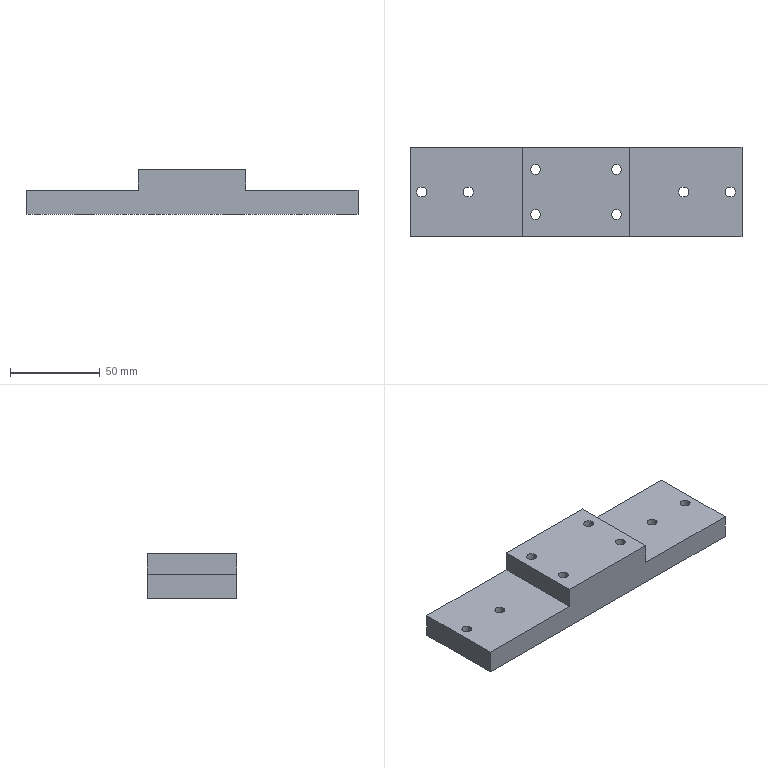Part | SolidWorks | features HoleWzd 2, Extrusion 1, ICE 1 | 1 solid | 50 faces | box 185 x 50 x 25 mm | volume 153218 mm3 | cylinder 32 | plane 18 | commonest cylinder face diameters 5.5 x16 10 x16
STEP:
#1=CARTESIAN_POINT('',(27.5,12.5,5.7));
#2=VERTEX_POINT('',#1);
#3=CARTESIAN_POINT('',(17.5,12.5,5.7));
#4=VERTEX_POINT('',#3);
#5=CARTESIAN_POINT('',(22.5,12.5,5.7));
#6=DIRECTION('',(0.,0.,-1.));
#7=DIRECTION('',(-1.,0.,0.));
#8=AXIS2_PLACEMENT_3D('',#5,#6,#7);
#9=CIRCLE('',#8,5.);
#10=EDGE_CURVE('',#2,#4,#9,.T.);
#11=ORIENTED_EDGE('',*,*,#10,.F.);
#12=CARTESIAN_POINT('',(27.5,12.5,0.));
#13=VERTEX_POINT('',#12);
#14=CARTESIAN_POINT('',(27.5,12.5,0.));
#15=DIRECTION('',(0.,0.,-1.));
#16=VECTOR('',#15,1000.);
#17=LINE('',#14,#16);
#18=EDGE_CURVE('',#2,#13,#17,.T.);
#19=ORIENTED_EDGE('',*,*,#18,.T.);
#20=CARTESIAN_POINT('',(17.5,12.5,0.));
#21=VERTEX_POINT('',#20);
#22=CARTESIAN_POINT('',(22.5,12.5,0.));
#23=DIRECTION('',(0.,0.,-1.));
#24=DIRECTION('',(-1.,0.,0.));
#25=AXIS2_PLACEMENT_3D('',#22,#23,#24);
#26=CIRCLE('',#25,5.);
#27=EDGE_CURVE('',#13,#21,#26,.T.);
#28=ORIENTED_EDGE('',*,*,#27,.T.);
#29=CARTESIAN_POINT('',(17.5,12.5,0.));
#30=DIRECTION('',(0.,0.,-1.));
#31=VECTOR('',#30,1000.);
#32=LINE('',#29,#31);
#33=EDGE_CURVE('',#4,#21,#32,.T.);
#34=ORIENTED_EDGE('',*,*,#33,.F.);
#35=EDGE_LOOP('',(#11,#19,#28,#34));
#36=FACE_OUTER_BOUND('',#35,.T.);
#37=CARTESIAN_POINT('',(22.5,12.5,0.));
#38=DIRECTION('',(0.,0.,-1.));
#39=DIRECTION('',(-1.,0.,0.));
#40=AXIS2_PLACEMENT_3D('',#37,#38,#39);
#41=CYLINDRICAL_SURFACE('',#40,5.);
#42=ADVANCED_FACE('',(#36),#41,.F.);
#43=CARTESIAN_POINT('',(25.25,12.5,25.));
#44=VERTEX_POINT('',#43);
#45=CARTESIAN_POINT('',(19.75,12.5,25.));
#46=VERTEX_POINT('',#45);
#47=CARTESIAN_POINT('',(22.5,12.5,25.));
#48=DIRECTION('',(0.,0.,-1.));
#49=DIRECTION('',(-1.,0.,0.));
#50=AXIS2_PLACEMENT_3D('',#47,#48,#49);
#51=CIRCLE('',#50,2.75);
#52=EDGE_CURVE('',#44,#46,#51,.T.);
#53=ORIENTED_EDGE('',*,*,#52,.F.);
#54=CARTESIAN_POINT('',(25.25,12.5,5.7));
#55=VERTEX_POINT('',#54);
#56=CARTESIAN_POINT('',(25.25,12.5,0.));
#57=DIRECTION('',(0.,0.,-1.));
#58=VECTOR('',#57,1000.);
#59=LINE('',#56,#58);
#60=EDGE_CURVE('',#44,#55,#59,.T.);
#61=ORIENTED_EDGE('',*,*,#60,.T.);
#62=CARTESIAN_POINT('',(19.75,12.5,5.7));
#63=VERTEX_POINT('',#62);
#64=CARTESIAN_POINT('',(22.5,12.5,5.7));
#65=DIRECTION('',(0.,0.,-1.));
#66=DIRECTION('',(-1.,0.,0.));
#67=AXIS2_PLACEMENT_3D('',#64,#65,#66);
#68=CIRCLE('',#67,2.75);
#69=EDGE_CURVE('',#55,#63,#68,.T.);
#70=ORIENTED_EDGE('',*,*,#69,.T.);
#71=CARTESIAN_POINT('',(19.75,12.5,0.));
#72=DIRECTION('',(0.,0.,-1.));
#73=VECTOR('',#72,1000.);
#74=LINE('',#71,#73);
#75=EDGE_CURVE('',#46,#63,#74,.T.);
#76=ORIENTED_EDGE('',*,*,#75,.F.);
#77=EDGE_LOOP('',(#53,#61,#70,#76));
#78=FACE_OUTER_BOUND('',#77,.T.);
#79=CARTESIAN_POINT('',(22.5,12.5,0.));
#80=DIRECTION('',(0.,0.,-1.));
#81=DIRECTION('',(-1.,0.,0.));
#82=AXIS2_PLACEMENT_3D('',#79,#80,#81);
#83=CYLINDRICAL_SURFACE('',#82,2.75);
#84=ADVANCED_FACE('',(#78),#83,.F.);
#85=CARTESIAN_POINT('',(27.5,-12.5,5.7));
#86=VERTEX_POINT('',#85);
#87=CARTESIAN_POINT('',(17.5,-12.5,5.7));
#88=VERTEX_POINT('',#87);
#89=CARTESIAN_POINT('',(22.5,-12.5,5.7));
#90=DIRECTION('',(0.,0.,-1.));
#91=DIRECTION('',(-1.,0.,0.));
#92=AXIS2_PLACEMENT_3D('',#89,#90,#91);
#93=CIRCLE('',#92,5.);
#94=EDGE_CURVE('',#86,#88,#93,.T.);
#95=ORIENTED_EDGE('',*,*,#94,.F.);
#96=CARTESIAN_POINT('',(27.5,-12.5,0.));
#97=VERTEX_POINT('',#96);
#98=CARTESIAN_POINT('',(27.5,-12.5,0.));
#99=DIRECTION('',(0.,0.,-1.));
#100=VECTOR('',#99,1000.);
#101=LINE('',#98,#100);
#102=EDGE_CURVE('',#86,#97,#101,.T.);
#103=ORIENTED_EDGE('',*,*,#102,.T.);
#104=CARTESIAN_POINT('',(17.5,-12.5,0.));
#105=VERTEX_POINT('',#104);
#106=CARTESIAN_POINT('',(22.5,-12.5,0.));
#107=DIRECTION('',(0.,0.,-1.));
#108=DIRECTION('',(-1.,0.,0.));
#109=AXIS2_PLACEMENT_3D('',#106,#107,#108);
#110=CIRCLE('',#109,5.);
#111=EDGE_CURVE('',#97,#105,#110,.T.);
#112=ORIENTED_EDGE('',*,*,#111,.T.);
#113=CARTESIAN_POINT('',(17.5,-12.5,0.));
#114=DIRECTION('',(0.,0.,-1.));
#115=VECTOR('',#114,1000.);
#116=LINE('',#113,#115);
#117=EDGE_CURVE('',#88,#105,#116,.T.);
#118=ORIENTED_EDGE('',*,*,#117,.F.);
#119=EDGE_LOOP('',(#95,#103,#112,#118));
#120=FACE_OUTER_BOUND('',#119,.T.);
#121=CARTESIAN_POINT('',(22.5,-12.5,0.));
#122=DIRECTION('',(0.,0.,-1.));
#123=DIRECTION('',(-1.,0.,0.));
#124=AXIS2_PLACEMENT_3D('',#121,#122,#123);
#125=CYLINDRICAL_SURFACE('',#124,5.);
#126=ADVANCED_FACE('',(#120),#125,.F.);
#127=CARTESIAN_POINT('',(25.25,-12.5,25.));
#128=VERTEX_POINT('',#127);
#129=CARTESIAN_POINT('',(19.75,-12.5,25.));
#130=VERTEX_POINT('',#129);
#131=CARTESIAN_POINT('',(22.5,-12.5,25.));
#132=DIRECTION('',(0.,0.,-1.));
#133=DIRECTION('',(-1.,0.,0.));
#134=AXIS2_PLACEMENT_3D('',#131,#132,#133);
#135=CIRCLE('',#134,2.75);
#136=EDGE_CURVE('',#128,#130,#135,.T.);
#137=ORIENTED_EDGE('',*,*,#136,.F.);
#138=CARTESIAN_POINT('',(25.25,-12.5,5.7));
#139=VERTEX_POINT('',#138);
#140=CARTESIAN_POINT('',(25.25,-12.5,0.));
#141=DIRECTION('',(0.,0.,-1.));
#142=VECTOR('',#141,1000.);
#143=LINE('',#140,#142);
#144=EDGE_CURVE('',#128,#139,#143,.T.);
#145=ORIENTED_EDGE('',*,*,#144,.T.);
#146=CARTESIAN_POINT('',(19.75,-12.5,5.7));
#147=VERTEX_POINT('',#146);
#148=CARTESIAN_POINT('',(22.5,-12.5,5.7));
#149=DIRECTION('',(0.,0.,-1.));
#150=DIRECTION('',(-1.,0.,0.));
#151=AXIS2_PLACEMENT_3D('',#148,#149,#150);
#152=CIRCLE('',#151,2.75);
#153=EDGE_CURVE('',#139,#147,#152,.T.);
#154=ORIENTED_EDGE('',*,*,#153,.T.);
#155=CARTESIAN_POINT('',(19.75,-12.5,0.));
#156=DIRECTION('',(0.,0.,-1.));
#157=VECTOR('',#156,1000.);
#158=LINE('',#155,#157);
#159=EDGE_CURVE('',#130,#147,#158,.T.);
#160=ORIENTED_EDGE('',*,*,#159,.F.);
#161=EDGE_LOOP('',(#137,#145,#154,#160));
#162=FACE_OUTER_BOUND('',#161,.T.);
#163=CARTESIAN_POINT('',(22.5,-12.5,0.));
#164=DIRECTION('',(0.,0.,-1.));
#165=DIRECTION('',(-1.,0.,0.));
#166=AXIS2_PLACEMENT_3D('',#163,#164,#165);
#167=CYLINDRICAL_SURFACE('',#166,2.75);
#168=ADVANCED_FACE('',(#162),#167,.F.);
#169=CARTESIAN_POINT('',(-17.5,12.5,5.7));
#170=VERTEX_POINT('',#169);
#171=CARTESIAN_POINT('',(-27.5,12.5,5.7));
#172=VERTEX_POINT('',#171);
#173=CARTESIAN_POINT('',(-22.5,12.5,5.7));
#174=DIRECTION('',(0.,0.,-1.));
#175=DIRECTION('',(-1.,0.,0.));
#176=AXIS2_PLACEMENT_3D('',#173,#174,#175);
#177=CIRCLE('',#176,5.);
#178=EDGE_CURVE('',#170,#172,#177,.T.);
#179=ORIENTED_EDGE('',*,*,#178,.F.);
#180=CARTESIAN_POINT('',(-17.5,12.5,0.));
#181=VERTEX_POINT('',#180);
#182=CARTESIAN_POINT('',(-17.5,12.5,0.));
#183=DIRECTION('',(0.,0.,-1.));
#184=VECTOR('',#183,1000.);
#185=LINE('',#182,#184);
#186=EDGE_CURVE('',#170,#181,#185,.T.);
#187=ORIENTED_EDGE('',*,*,#186,.T.);
#188=CARTESIAN_POINT('',(-27.5,12.5,0.));
#189=VERTEX_POINT('',#188);
#190=CARTESIAN_POINT('',(-22.5,12.5,0.));
#191=DIRECTION('',(0.,0.,-1.));
#192=DIRECTION('',(-1.,0.,0.));
#193=AXIS2_PLACEMENT_3D('',#190,#191,#192);
#194=CIRCLE('',#193,5.);
#195=EDGE_CURVE('',#181,#189,#194,.T.);
#196=ORIENTED_EDGE('',*,*,#195,.T.);
#197=CARTESIAN_POINT('',(-27.5,12.5,0.));
#198=DIRECTION('',(0.,0.,-1.));
#199=VECTOR('',#198,1000.);
#200=LINE('',#197,#199);
#201=EDGE_CURVE('',#172,#189,#200,.T.);
#202=ORIENTED_EDGE('',*,*,#201,.F.);
#203=EDGE_LOOP('',(#179,#187,#196,#202));
#204=FACE_OUTER_BOUND('',#203,.T.);
#205=CARTESIAN_POINT('',(-22.5,12.5,0.));
#206=DIRECTION('',(0.,0.,-1.));
#207=DIRECTION('',(-1.,0.,0.));
#208=AXIS2_PLACEMENT_3D('',#205,#206,#207);
#209=CYLINDRICAL_SURFACE('',#208,5.);
#210=ADVANCED_FACE('',(#204),#209,.F.);
#211=CARTESIAN_POINT('',(-19.75,12.5,25.));
#212=VERTEX_POINT('',#211);
#213=CARTESIAN_POINT('',(-25.25,12.5,25.));
#214=VERTEX_POINT('',#213);
#215=CARTESIAN_POINT('',(-22.5,12.5,25.));
#216=DIRECTION('',(0.,0.,-1.));
#217=DIRECTION('',(-1.,0.,0.));
#218=AXIS2_PLACEMENT_3D('',#215,#216,#217);
#219=CIRCLE('',#218,2.75);
#220=EDGE_CURVE('',#212,#214,#219,.T.);
#221=ORIENTED_EDGE('',*,*,#220,.F.);
#222=CARTESIAN_POINT('',(-19.75,12.5,5.7));
#223=VERTEX_POINT('',#222);
#224=CARTESIAN_POINT('',(-19.75,12.5,0.));
#225=DIRECTION('',(0.,0.,-1.));
#226=VECTOR('',#225,1000.);
#227=LINE('',#224,#226);
#228=EDGE_CURVE('',#212,#223,#227,.T.);
#229=ORIENTED_EDGE('',*,*,#228,.T.);
#230=CARTESIAN_POINT('',(-25.25,12.5,5.7));
#231=VERTEX_POINT('',#230);
#232=CARTESIAN_POINT('',(-22.5,12.5,5.7));
#233=DIRECTION('',(0.,0.,-1.));
#234=DIRECTION('',(-1.,0.,0.));
#235=AXIS2_PLACEMENT_3D('',#232,#233,#234);
#236=CIRCLE('',#235,2.75);
#237=EDGE_CURVE('',#223,#231,#236,.T.);
#238=ORIENTED_EDGE('',*,*,#237,.T.);
#239=CARTESIAN_POINT('',(-25.25,12.5,0.));
#240=DIRECTION('',(0.,0.,-1.));
#241=VECTOR('',#240,1000.);
#242=LINE('',#239,#241);
#243=EDGE_CURVE('',#214,#231,#242,.T.);
#244=ORIENTED_EDGE('',*,*,#243,.F.);
#245=EDGE_LOOP('',(#221,#229,#238,#244));
#246=FACE_OUTER_BOUND('',#245,.T.);
#247=CARTESIAN_POINT('',(-22.5,12.5,0.));
#248=DIRECTION('',(0.,0.,-1.));
#249=DIRECTION('',(-1.,0.,0.));
#250=AXIS2_PLACEMENT_3D('',#247,#248,#249);
#251=CYLINDRICAL_SURFACE('',#250,2.75);
#252=ADVANCED_FACE('',(#246),#251,.F.);
#253=CARTESIAN_POINT('',(-17.5,-12.5,5.7));
#254=VERTEX_POINT('',#253);
#255=CARTESIAN_POINT('',(-27.5,-12.5,5.7));
#256=VERTEX_POINT('',#255);
#257=CARTESIAN_POINT('',(-22.5,-12.5,5.7));
#258=DIRECTION('',(0.,0.,-1.));
#259=DIRECTION('',(-1.,0.,0.));
#260=AXIS2_PLACEMENT_3D('',#257,#258,#259);
#261=CIRCLE('',#260,5.);
#262=EDGE_CURVE('',#254,#256,#261,.T.);
#263=ORIENTED_EDGE('',*,*,#262,.F.);
#264=CARTESIAN_POINT('',(-17.5,-12.5,0.));
#265=VERTEX_POINT('',#264);
#266=CARTESIAN_POINT('',(-17.5,-12.5,0.));
#267=DIRECTION('',(0.,0.,-1.));
#268=VECTOR('',#267,1000.);
#269=LINE('',#266,#268);
#270=EDGE_CURVE('',#254,#265,#269,.T.);
#271=ORIENTED_EDGE('',*,*,#270,.T.);
#272=CARTESIAN_POINT('',(-27.5,-12.5,0.));
#273=VERTEX_POINT('',#272);
#274=CARTESIAN_POINT('',(-22.5,-12.5,0.));
#275=DIRECTION('',(0.,0.,-1.));
#276=DIRECTION('',(-1.,0.,0.));
#277=AXIS2_PLACEMENT_3D('',#274,#275,#276);
#278=CIRCLE('',#277,5.);
#279=EDGE_CURVE('',#265,#273,#278,.T.);
#280=ORIENTED_EDGE('',*,*,#279,.T.);
#281=CARTESIAN_POINT('',(-27.5,-12.5,0.));
#282=DIRECTION('',(0.,0.,-1.));
#283=VECTOR('',#282,1000.);
#284=LINE('',#281,#283);
#285=EDGE_CURVE('',#256,#273,#284,.T.);
#286=ORIENTED_EDGE('',*,*,#285,.F.);
#287=EDGE_LOOP('',(#263,#271,#280,#286));
#288=FACE_OUTER_BOUND('',#287,.T.);
#289=CARTESIAN_POINT('',(-22.5,-12.5,0.));
#290=DIRECTION('',(0.,0.,-1.));
#291=DIRECTION('',(-1.,0.,0.));
#292=AXIS2_PLACEMENT_3D('',#289,#290,#291);
#293=CYLINDRICAL_SURFACE('',#292,5.);
#294=ADVANCED_FACE('',(#288),#293,.F.);
#295=CARTESIAN_POINT('',(-19.75,-12.5,25.));
#296=VERTEX_POINT('',#295);
#297=CARTESIAN_POINT('',(-25.25,-12.5,25.));
#298=VERTEX_POINT('',#297);
#299=CARTESIAN_POINT('',(-22.5,-12.5,25.));
#300=DIRECTION('',(0.,0.,-1.));
#301=DIRECTION('',(-1.,0.,0.));
#302=AXIS2_PLACEMENT_3D('',#299,#300,#301);
#303=CIRCLE('',#302,2.75);
#304=EDGE_CURVE('',#296,#298,#303,.T.);
#305=ORIENTED_EDGE('',*,*,#304,.F.);
#306=CARTESIAN_POINT('',(-19.75,-12.5,5.7));
#307=VERTEX_POINT('',#306);
#308=CARTESIAN_POINT('',(-19.75,-12.5,0.));
#309=DIRECTION('',(0.,0.,-1.));
#310=VECTOR('',#309,1000.);
#311=LINE('',#308,#310);
#312=EDGE_CURVE('',#296,#307,#311,.T.);
#313=ORIENTED_EDGE('',*,*,#312,.T.);
#314=CARTESIAN_POINT('',(-25.25,-12.5,5.7));
#315=VERTEX_POINT('',#314);
#316=CARTESIAN_POINT('',(-22.5,-12.5,5.7));
#317=DIRECTION('',(0.,0.,-1.));
#318=DIRECTION('',(-1.,0.,0.));
#319=AXIS2_PLACEMENT_3D('',#316,#317,#318);
#320=CIRCLE('',#319,2.75);
#321=EDGE_CURVE('',#307,#315,#320,.T.);
#322=ORIENTED_EDGE('',*,*,#321,.T.);
#323=CARTESIAN_POINT('',(-25.25,-12.5,0.));
#324=DIRECTION('',(0.,0.,-1.));
#325=VECTOR('',#324,1000.);
#326=LINE('',#323,#325);
#327=EDGE_CURVE('',#298,#315,#326,.T.);
#328=ORIENTED_EDGE('',*,*,#327,.F.);
#329=EDGE_LOOP('',(#305,#313,#322,#328));
#330=FACE_OUTER_BOUND('',#329,.T.);
#331=CARTESIAN_POINT('',(-22.5,-12.5,0.));
#332=DIRECTION('',(0.,0.,-1.));
#333=DIRECTION('',(-1.,0.,0.));
#334=AXIS2_PLACEMENT_3D('',#331,#332,#333);
#335=CYLINDRICAL_SURFACE('',#334,2.75);
#336=ADVANCED_FACE('',(#330),#335,.F.);
#337=CARTESIAN_POINT('',(91.,0.,5.7));
#338=VERTEX_POINT('',#337);
#339=CARTESIAN_POINT('',(81.,0.,5.7));
#340=VERTEX_POINT('',#339);
#341=CARTESIAN_POINT('',(86.,0.,5.7));
#342=DIRECTION('',(0.,0.,-1.));
#343=DIRECTION('',(-1.,0.,0.));
#344=AXIS2_PLACEMENT_3D('',#341,#342,#343);
#345=CIRCLE('',#344,5.);
#346=EDGE_CURVE('',#338,#340,#345,.T.);
#347=ORIENTED_EDGE('',*,*,#346,.F.);
#348=CARTESIAN_POINT('',(91.,0.,0.));
#349=VERTEX_POINT('',#348);
#350=CARTESIAN_POINT('',(91.,0.,0.));
#351=DIRECTION('',(0.,0.,-1.));
#352=VECTOR('',#351,1000.);
#353=LINE('',#350,#352);
#354=EDGE_CURVE('',#338,#349,#353,.T.);
#355=ORIENTED_EDGE('',*,*,#354,.T.);
#356=CARTESIAN_POINT('',(81.,0.,0.));
#357=VERTEX_POINT('',#356);
#358=CARTESIAN_POINT('',(86.,0.,0.));
#359=DIRECTION('',(0.,0.,-1.));
#360=DIRECTION('',(-1.,0.,0.));
#361=AXIS2_PLACEMENT_3D('',#358,#359,#360);
#362=CIRCLE('',#361,5.);
#363=EDGE_CURVE('',#349,#357,#362,.T.);
#364=ORIENTED_EDGE('',*,*,#363,.T.);
#365=CARTESIAN_POINT('',(81.,0.,0.));
#366=DIRECTION('',(0.,0.,-1.));
#367=VECTOR('',#366,1000.);
#368=LINE('',#365,#367);
#369=EDGE_CURVE('',#340,#357,#368,.T.);
#370=ORIENTED_EDGE('',*,*,#369,.F.);
#371=EDGE_LOOP('',(#347,#355,#364,#370));
#372=FACE_OUTER_BOUND('',#371,.T.);
#373=CARTESIAN_POINT('',(86.,0.,0.));
#374=DIRECTION('',(0.,0.,-1.));
#375=DIRECTION('',(-1.,0.,0.));
#376=AXIS2_PLACEMENT_3D('',#373,#374,#375);
#377=CYLINDRICAL_SURFACE('',#376,5.);
#378=ADVANCED_FACE('',(#372),#377,.F.);
#379=CARTESIAN_POINT('',(88.75,0.,13.5));
#380=VERTEX_POINT('',#379);
#381=CARTESIAN_POINT('',(83.25,0.,13.5));
#382=VERTEX_POINT('',#381);
#383=CARTESIAN_POINT('',(86.,0.,13.5));
#384=DIRECTION('',(0.,0.,-1.));
#385=DIRECTION('',(-1.,0.,0.));
#386=AXIS2_PLACEMENT_3D('',#383,#384,#385);
#387=CIRCLE('',#386,2.75);
#388=EDGE_CURVE('',#380,#382,#387,.T.);
#389=ORIENTED_EDGE('',*,*,#388,.F.);
#390=CARTESIAN_POINT('',(88.75,0.,5.7));
#391=VERTEX_POINT('',#390);
#392=CARTESIAN_POINT('',(88.75,0.,0.));
#393=DIRECTION('',(0.,0.,-1.));
#394=VECTOR('',#393,1000.);
#395=LINE('',#392,#394);
#396=EDGE_CURVE('',#380,#391,#395,.T.);
#397=ORIENTED_EDGE('',*,*,#396,.T.);
#398=CARTESIAN_POINT('',(83.25,0.,5.7));
#399=VERTEX_POINT('',#398);
#400=CARTESIAN_POINT('',(86.,0.,5.7));
#401=DIRECTION('',(0.,0.,-1.));
#402=DIRECTION('',(-1.,0.,0.));
#403=AXIS2_PLACEMENT_3D('',#400,#401,#402);
#404=CIRCLE('',#403,2.75);
#405=EDGE_CURVE('',#391,#399,#404,.T.);
#406=ORIENTED_EDGE('',*,*,#405,.T.);
#407=CARTESIAN_POINT('',(83.25,0.,0.));
#408=DIRECTION('',(0.,0.,-1.));
#409=VECTOR('',#408,1000.);
#410=LINE('',#407,#409);
#411=EDGE_CURVE('',#382,#399,#410,.T.);
#412=ORIENTED_EDGE('',*,*,#411,.F.);
#413=EDGE_LOOP('',(#389,#397,#406,#412));
#414=FACE_OUTER_BOUND('',#413,.T.);
#415=CARTESIAN_POINT('',(86.,0.,0.));
#416=DIRECTION('',(0.,0.,-1.));
#417=DIRECTION('',(-1.,0.,0.));
#418=AXIS2_PLACEMENT_3D('',#415,#416,#417);
#419=CYLINDRICAL_SURFACE('',#418,2.75);
#420=ADVANCED_FACE('',(#414),#419,.F.);
#421=CARTESIAN_POINT('',(65.,0.,5.7));
#422=VERTEX_POINT('',#421);
#423=CARTESIAN_POINT('',(55.,0.,5.7));
#424=VERTEX_POINT('',#423);
#425=CARTESIAN_POINT('',(60.,0.,5.7));
#426=DIRECTION('',(0.,0.,-1.));
#427=DIRECTION('',(-1.,0.,0.));
#428=AXIS2_PLACEMENT_3D('',#425,#426,#427);
#429=CIRCLE('',#428,5.);
#430=EDGE_CURVE('',#422,#424,#429,.T.);
#431=ORIENTED_EDGE('',*,*,#430,.F.);
#432=CARTESIAN_POINT('',(65.,0.,0.));
#433=VERTEX_POINT('',#432);
#434=CARTESIAN_POINT('',(65.,0.,0.));
#435=DIRECTION('',(0.,0.,-1.));
#436=VECTOR('',#435,1000.);
#437=LINE('',#434,#436);
#438=EDGE_CURVE('',#422,#433,#437,.T.);
#439=ORIENTED_EDGE('',*,*,#438,.T.);
#440=CARTESIAN_POINT('',(55.,0.,0.));
#441=VERTEX_POINT('',#440);
#442=CARTESIAN_POINT('',(60.,0.,0.));
#443=DIRECTION('',(0.,0.,-1.));
#444=DIRECTION('',(-1.,0.,0.));
#445=AXIS2_PLACEMENT_3D('',#442,#443,#444);
#446=CIRCLE('',#445,5.);
#447=EDGE_CURVE('',#433,#441,#446,.T.);
#448=ORIENTED_EDGE('',*,*,#447,.T.);
#449=CARTESIAN_POINT('',(55.,0.,0.));
#450=DIRECTION('',(0.,0.,-1.));
#451=VECTOR('',#450,1000.);
#452=LINE('',#449,#451);
#453=EDGE_CURVE('',#424,#441,#452,.T.);
#454=ORIENTED_EDGE('',*,*,#453,.F.);
#455=EDGE_LOOP('',(#431,#439,#448,#454));
#456=FACE_OUTER_BOUND('',#455,.T.);
#457=CARTESIAN_POINT('',(60.,0.,0.));
#458=DIRECTION('',(0.,0.,-1.));
#459=DIRECTION('',(-1.,0.,0.));
#460=AXIS2_PLACEMENT_3D('',#457,#458,#459);
#461=CYLINDRICAL_SURFACE('',#460,5.);
#462=ADVANCED_FACE('',(#456),#461,.F.);
#463=CARTESIAN_POINT('',(62.75,0.,13.5));
#464=VERTEX_POINT('',#463);
#465=CARTESIAN_POINT('',(57.25,0.,13.5));
#466=VERTEX_POINT('',#465);
#467=CARTESIAN_POINT('',(60.,0.,13.5));
#468=DIRECTION('',(0.,0.,-1.));
#469=DIRECTION('',(-1.,0.,0.));
#470=AXIS2_PLACEMENT_3D('',#467,#468,#469);
#471=CIRCLE('',#470,2.75);
#472=EDGE_CURVE('',#464,#466,#471,.T.);
#473=ORIENTED_EDGE('',*,*,#472,.F.);
#474=CARTESIAN_POINT('',(62.75,0.,5.7));
#475=VERTEX_POINT('',#474);
#476=CARTESIAN_POINT('',(62.75,0.,0.));
#477=DIRECTION('',(0.,0.,-1.));
#478=VECTOR('',#477,1000.);
#479=LINE('',#476,#478);
#480=EDGE_CURVE('',#464,#475,#479,.T.);
#481=ORIENTED_EDGE('',*,*,#480,.T.);
#482=CARTESIAN_POINT('',(57.25,0.,5.7));
#483=VERTEX_POINT('',#482);
#484=CARTESIAN_POINT('',(60.,0.,5.7));
#485=DIRECTION('',(0.,0.,-1.));
#486=DIRECTION('',(-1.,0.,0.));
#487=AXIS2_PLACEMENT_3D('',#484,#485,#486);
#488=CIRCLE('',#487,2.75);
#489=EDGE_CURVE('',#475,#483,#488,.T.);
#490=ORIENTED_EDGE('',*,*,#489,.T.);
#491=CARTESIAN_POINT('',(57.25,0.,0.));
#492=DIRECTION('',(0.,0.,-1.));
#493=VECTOR('',#492,1000.);
#494=LINE('',#491,#493);
#495=EDGE_CURVE('',#466,#483,#494,.T.);
#496=ORIENTED_EDGE('',*,*,#495,.F.);
#497=EDGE_LOOP('',(#473,#481,#490,#496));
#498=FACE_OUTER_BOUND('',#497,.T.);
#499=CARTESIAN_POINT('',(60.,0.,0.));
#500=DIRECTION('',(0.,0.,-1.));
#501=DIRECTION('',(-1.,0.,0.));
#502=AXIS2_PLACEMENT_3D('',#499,#500,#501);
#503=CYLINDRICAL_SURFACE('',#502,2.75);
#504=ADVANCED_FACE('',(#498),#503,.F.);
#505=CARTESIAN_POINT('',(-55.,0.,5.7));
#506=VERTEX_POINT('',#505);
#507=CARTESIAN_POINT('',(-65.,0.,5.7));
#508=VERTEX_POINT('',#507);
#509=CARTESIAN_POINT('',(-60.,0.,5.7));
#510=DIRECTION('',(0.,0.,-1.));
#511=DIRECTION('',(-1.,0.,0.));
#512=AXIS2_PLACEMENT_3D('',#509,#510,#511);
#513=CIRCLE('',#512,5.);
#514=EDGE_CURVE('',#506,#508,#513,.T.);
#515=ORIENTED_EDGE('',*,*,#514,.F.);
#516=CARTESIAN_POINT('',(-55.,0.,0.));
#517=VERTEX_POINT('',#516);
#518=CARTESIAN_POINT('',(-55.,0.,0.));
#519=DIRECTION('',(0.,0.,-1.));
#520=VECTOR('',#519,1000.);
#521=LINE('',#518,#520);
#522=EDGE_CURVE('',#506,#517,#521,.T.);
#523=ORIENTED_EDGE('',*,*,#522,.T.);
#524=CARTESIAN_POINT('',(-65.,0.,0.));
#525=VERTEX_POINT('',#524);
#526=CARTESIAN_POINT('',(-60.,0.,0.));
#527=DIRECTION('',(0.,0.,-1.));
#528=DIRECTION('',(-1.,0.,0.));
#529=AXIS2_PLACEMENT_3D('',#526,#527,#528);
#530=CIRCLE('',#529,5.);
#531=EDGE_CURVE('',#517,#525,#530,.T.);
#532=ORIENTED_EDGE('',*,*,#531,.T.);
#533=CARTESIAN_POINT('',(-65.,0.,0.));
#534=DIRECTION('',(0.,0.,-1.));
#535=VECTOR('',#534,1000.);
#536=LINE('',#533,#535);
#537=EDGE_CURVE('',#508,#525,#536,.T.);
#538=ORIENTED_EDGE('',*,*,#537,.F.);
#539=EDGE_LOOP('',(#515,#523,#532,#538));
#540=FACE_OUTER_BOUND('',#539,.T.);
#541=CARTESIAN_POINT('',(-60.,0.,0.));
#542=DIRECTION('',(0.,0.,-1.));
#543=DIRECTION('',(-1.,0.,0.));
#544=AXIS2_PLACEMENT_3D('',#541,#542,#543);
#545=CYLINDRICAL_SURFACE('',#544,5.);
#546=ADVANCED_FACE('',(#540),#545,.F.);
#547=CARTESIAN_POINT('',(-62.75,0.,13.5));
#548=VERTEX_POINT('',#547);
#549=CARTESIAN_POINT('',(-57.25,0.,13.5));
#550=VERTEX_POINT('',#549);
#551=CARTESIAN_POINT('',(-60.,0.,13.5));
#552=DIRECTION('',(0.,0.,1.));
#553=DIRECTION('',(1.,0.,0.));
#554=AXIS2_PLACEMENT_3D('',#551,#552,#553);
#555=CIRCLE('',#554,2.75);
#556=EDGE_CURVE('',#548,#550,#555,.T.);
#557=ORIENTED_EDGE('',*,*,#556,.T.);
#558=CARTESIAN_POINT('',(-57.25,0.,5.7));
#559=VERTEX_POINT('',#558);
#560=CARTESIAN_POINT('',(-57.25,0.,0.));
#561=DIRECTION('',(0.,0.,-1.));
#562=VECTOR('',#561,1000.);
#563=LINE('',#560,#562);
#564=EDGE_CURVE('',#550,#559,#563,.T.);
#565=ORIENTED_EDGE('',*,*,#564,.T.);
#566=CARTESIAN_POINT('',(-62.75,0.,5.7));
#567=VERTEX_POINT('',#566);
#568=CARTESIAN_POINT('',(-60.,0.,5.7));
#569=DIRECTION('',(0.,0.,-1.));
#570=DIRECTION('',(-1.,0.,0.));
#571=AXIS2_PLACEMENT_3D('',#568,#569,#570);
#572=CIRCLE('',#571,2.75);
#573=EDGE_CURVE('',#559,#567,#572,.T.);
#574=ORIENTED_EDGE('',*,*,#573,.T.);
#575=CARTESIAN_POINT('',(-62.75,0.,0.));
#576=DIRECTION('',(0.,0.,-1.));
#577=VECTOR('',#576,1000.);
#578=LINE('',#575,#577);
#579=EDGE_CURVE('',#548,#567,#578,.T.);
#580=ORIENTED_EDGE('',*,*,#579,.F.);
#581=EDGE_LOOP('',(#557,#565,#574,#580));
#582=FACE_OUTER_BOUND('',#581,.T.);
#583=CARTESIAN_POINT('',(-60.,0.,0.));
#584=DIRECTION('',(0.,0.,-1.));
#585=DIRECTION('',(-1.,0.,0.));
#586=AXIS2_PLACEMENT_3D('',#583,#584,#585);
#587=CYLINDRICAL_SURFACE('',#586,2.75);
#588=ADVANCED_FACE('',(#582),#587,.F.);
#589=CARTESIAN_POINT('',(-81.,0.,5.7));
#590=VERTEX_POINT('',#589);
#591=CARTESIAN_POINT('',(-91.,0.,5.7));
#592=VERTEX_POINT('',#591);
#593=CARTESIAN_POINT('',(-86.,0.,5.7));
#594=DIRECTION('',(0.,0.,-1.));
#595=DIRECTION('',(-1.,0.,0.));
#596=AXIS2_PLACEMENT_3D('',#593,#594,#595);
#597=CIRCLE('',#596,5.);
#598=EDGE_CURVE('',#590,#592,#597,.T.);
#599=ORIENTED_EDGE('',*,*,#598,.F.);
#600=CARTESIAN_POINT('',(-81.,0.,0.));
#601=VERTEX_POINT('',#600);
#602=CARTESIAN_POINT('',(-81.,0.,0.));
#603=DIRECTION('',(0.,0.,-1.));
#604=VECTOR('',#603,1000.);
#605=LINE('',#602,#604);
#606=EDGE_CURVE('',#590,#601,#605,.T.);
#607=ORIENTED_EDGE('',*,*,#606,.T.);
#608=CARTESIAN_POINT('',(-91.,0.,0.));
#609=VERTEX_POINT('',#608);
#610=CARTESIAN_POINT('',(-86.,0.,0.));
#611=DIRECTION('',(0.,0.,-1.));
#612=DIRECTION('',(-1.,0.,0.));
#613=AXIS2_PLACEMENT_3D('',#610,#611,#612);
#614=CIRCLE('',#613,5.);
#615=EDGE_CURVE('',#601,#609,#614,.T.);
#616=ORIENTED_EDGE('',*,*,#615,.T.);
#617=CARTESIAN_POINT('',(-91.,0.,0.));
#618=DIRECTION('',(0.,0.,-1.));
#619=VECTOR('',#618,1000.);
#620=LINE('',#617,#619);
#621=EDGE_CURVE('',#592,#609,#620,.T.);
#622=ORIENTED_EDGE('',*,*,#621,.F.);
#623=EDGE_LOOP('',(#599,#607,#616,#622));
#624=FACE_OUTER_BOUND('',#623,.T.);
#625=CARTESIAN_POINT('',(-86.,0.,0.));
#626=DIRECTION('',(0.,0.,-1.));
#627=DIRECTION('',(-1.,0.,0.));
#628=AXIS2_PLACEMENT_3D('',#625,#626,#627);
#629=CYLINDRICAL_SURFACE('',#628,5.);
#630=ADVANCED_FACE('',(#624),#629,.F.);
#631=CARTESIAN_POINT('',(-88.75,0.,13.5));
#632=VERTEX_POINT('',#631);
#633=CARTESIAN_POINT('',(-83.25,0.,13.5));
#634=VERTEX_POINT('',#633);
#635=CARTESIAN_POINT('',(-86.,0.,13.5));
#636=DIRECTION('',(0.,0.,1.));
#637=DIRECTION('',(1.,0.,0.));
#638=AXIS2_PLACEMENT_3D('',#635,#636,#637);
#639=CIRCLE('',#638,2.75);
#640=EDGE_CURVE('',#632,#634,#639,.T.);
#641=ORIENTED_EDGE('',*,*,#640,.T.);
#642=CARTESIAN_POINT('',(-83.25,0.,5.7));
#643=VERTEX_POINT('',#642);
#644=CARTESIAN_POINT('',(-83.25,0.,0.));
#645=DIRECTION('',(0.,0.,-1.));
#646=VECTOR('',#645,1000.);
#647=LINE('',#644,#646);
#648=EDGE_CURVE('',#634,#643,#647,.T.);
#649=ORIENTED_EDGE('',*,*,#648,.T.);
#650=CARTESIAN_POINT('',(-88.75,0.,5.7));
#651=VERTEX_POINT('',#650);
#652=CARTESIAN_POINT('',(-86.,0.,5.7));
#653=DIRECTION('',(0.,0.,-1.));
#654=DIRECTION('',(-1.,0.,0.));
#655=AXIS2_PLACEMENT_3D('',#652,#653,#654);
#656=CIRCLE('',#655,2.75);
#657=EDGE_CURVE('',#643,#651,#656,.T.);
#658=ORIENTED_EDGE('',*,*,#657,.T.);
#659=CARTESIAN_POINT('',(-88.75,0.,0.));
#660=DIRECTION('',(0.,0.,-1.));
#661=VECTOR('',#660,1000.);
#662=LINE('',#659,#661);
#663=EDGE_CURVE('',#632,#651,#662,.T.);
#664=ORIENTED_EDGE('',*,*,#663,.F.);
#665=EDGE_LOOP('',(#641,#649,#658,#664));
#666=FACE_OUTER_BOUND('',#665,.T.);
#667=CARTESIAN_POINT('',(-86.,0.,0.));
#668=DIRECTION('',(0.,0.,-1.));
#669=DIRECTION('',(-1.,0.,0.));
#670=AXIS2_PLACEMENT_3D('',#667,#668,#669);
#671=CYLINDRICAL_SURFACE('',#670,2.75);
#672=ADVANCED_FACE('',(#666),#671,.F.);
#673=CARTESIAN_POINT('',(-92.5,25.,13.5));
#674=VERTEX_POINT('',#673);
#675=CARTESIAN_POINT('',(-92.5,-25.,13.5));
#676=VERTEX_POINT('',#675);
#677=CARTESIAN_POINT('',(-92.5,25.,13.5));
#678=DIRECTION('',(0.,-1.,0.));
#679=VECTOR('',#678,1000.);
#680=LINE('',#677,#679);
#681=EDGE_CURVE('',#674,#676,#680,.T.);
#682=ORIENTED_EDGE('',*,*,#681,.F.);
#683=CARTESIAN_POINT('',(-92.5,25.,0.));
#684=VERTEX_POINT('',#683);
#685=CARTESIAN_POINT('',(-92.5,25.,25.));
#686=DIRECTION('',(0.,0.,-1.));
#687=VECTOR('',#686,1000.);
#688=LINE('',#685,#687);
#689=EDGE_CURVE('',#674,#684,#688,.T.);
#690=ORIENTED_EDGE('',*,*,#689,.T.);
#691=CARTESIAN_POINT('',(-92.5,-25.,0.));
#692=VERTEX_POINT('',#691);
#693=CARTESIAN_POINT('',(-92.5,25.,0.));
#694=DIRECTION('',(0.,-1.,0.));
#695=VECTOR('',#694,1000.);
#696=LINE('',#693,#695);
#697=EDGE_CURVE('',#684,#692,#696,.T.);
#698=ORIENTED_EDGE('',*,*,#697,.T.);
#699=CARTESIAN_POINT('',(-92.5,-25.,25.));
#700=DIRECTION('',(0.,0.,-1.));
#701=VECTOR('',#700,1000.);
#702=LINE('',#699,#701);
#703=EDGE_CURVE('',#676,#692,#702,.T.);
#704=ORIENTED_EDGE('',*,*,#703,.F.);
#705=EDGE_LOOP('',(#682,#690,#698,#704));
#706=FACE_OUTER_BOUND('',#705,.T.);
#707=CARTESIAN_POINT('',(-92.5,25.,25.));
#708=DIRECTION('',(1.,0.,0.));
#709=DIRECTION('',(0.,0.,-1.));
#710=AXIS2_PLACEMENT_3D('',#707,#708,#709);
#711=PLANE('',#710);
#712=ADVANCED_FACE('',(#706),#711,.F.);
#713=CARTESIAN_POINT('',(30.,-25.,13.5));
#714=VERTEX_POINT('',#713);
#715=CARTESIAN_POINT('',(92.5,-25.,13.5));
#716=VERTEX_POINT('',#715);
#717=CARTESIAN_POINT('',(92.5,-25.,13.5));
#718=DIRECTION('',(1.,0.,0.));
#719=VECTOR('',#718,1000.);
#720=LINE('',#717,#719);
#721=EDGE_CURVE('',#714,#716,#720,.T.);
#722=ORIENTED_EDGE('',*,*,#721,.F.);
#723=CARTESIAN_POINT('',(30.,-25.,25.));
#724=VERTEX_POINT('',#723);
#725=CARTESIAN_POINT('',(30.,-25.,13.5));
#726=DIRECTION('',(0.,0.,1.));
#727=VECTOR('',#726,1000.);
#728=LINE('',#725,#727);
#729=EDGE_CURVE('',#714,#724,#728,.T.);
#730=ORIENTED_EDGE('',*,*,#729,.T.);
#731=CARTESIAN_POINT('',(-30.,-25.,25.));
#732=VERTEX_POINT('',#731);
#733=CARTESIAN_POINT('',(-92.5,-25.,25.));
#734=DIRECTION('',(1.,0.,0.));
#735=VECTOR('',#734,1000.);
#736=LINE('',#733,#735);
#737=EDGE_CURVE('',#732,#724,#736,.T.);
#738=ORIENTED_EDGE('',*,*,#737,.F.);
#739=CARTESIAN_POINT('',(-30.,-25.,13.5));
#740=VERTEX_POINT('',#739);
#741=CARTESIAN_POINT('',(-30.,-25.,13.5));
#742=DIRECTION('',(0.,0.,1.));
#743=VECTOR('',#742,1000.);
#744=LINE('',#741,#743);
#745=EDGE_CURVE('',#740,#732,#744,.T.);
#746=ORIENTED_EDGE('',*,*,#745,.F.);
#747=CARTESIAN_POINT('',(-92.5,-25.,13.5));
#748=DIRECTION('',(1.,0.,0.));
#749=VECTOR('',#748,1000.);
#750=LINE('',#747,#749);
#751=EDGE_CURVE('',#676,#740,#750,.T.);
#752=ORIENTED_EDGE('',*,*,#751,.F.);
#753=ORIENTED_EDGE('',*,*,#703,.T.);
#754=CARTESIAN_POINT('',(92.5,-25.,0.));
#755=VERTEX_POINT('',#754);
#756=CARTESIAN_POINT('',(-92.5,-25.,0.));
#757=DIRECTION('',(1.,0.,0.));
#758=VECTOR('',#757,1000.);
#759=LINE('',#756,#758);
#760=EDGE_CURVE('',#692,#755,#759,.T.);
#761=ORIENTED_EDGE('',*,*,#760,.T.);
#762=CARTESIAN_POINT('',(92.5,-25.,25.));
#763=DIRECTION('',(0.,0.,-1.));
#764=VECTOR('',#763,1000.);
#765=LINE('',#762,#764);
#766=EDGE_CURVE('',#716,#755,#765,.T.);
#767=ORIENTED_EDGE('',*,*,#766,.F.);
#768=EDGE_LOOP('',(#722,#730,#738,#746,#752,#753,#761,#767));
#769=FACE_OUTER_BOUND('',#768,.T.);
#770=CARTESIAN_POINT('',(-92.5,-25.,25.));
#771=DIRECTION('',(0.,1.,0.));
#772=DIRECTION('',(0.,0.,1.));
#773=AXIS2_PLACEMENT_3D('',#770,#771,#772);
#774=PLANE('',#773);
#775=ADVANCED_FACE('',(#769),#774,.F.);
#776=CARTESIAN_POINT('',(92.5,25.,13.5));
#777=VERTEX_POINT('',#776);
#778=CARTESIAN_POINT('',(92.5,25.,0.));
#779=VERTEX_POINT('',#778);
#780=CARTESIAN_POINT('',(92.5,25.,25.));
#781=DIRECTION('',(0.,0.,-1.));
#782=VECTOR('',#781,1000.);
#783=LINE('',#780,#782);
#784=EDGE_CURVE('',#777,#779,#783,.T.);
#785=ORIENTED_EDGE('',*,*,#784,.F.);
#786=CARTESIAN_POINT('',(92.5,25.,13.5));
#787=DIRECTION('',(0.,1.,0.));
#788=VECTOR('',#787,1000.);
#789=LINE('',#786,#788);
#790=EDGE_CURVE('',#716,#777,#789,.T.);
#791=ORIENTED_EDGE('',*,*,#790,.F.);
#792=ORIENTED_EDGE('',*,*,#766,.T.);
#793=CARTESIAN_POINT('',(92.5,25.,0.));
#794=DIRECTION('',(0.,1.,0.));
#795=VECTOR('',#794,1000.);
#796=LINE('',#793,#795);
#797=EDGE_CURVE('',#755,#779,#796,.T.);
#798=ORIENTED_EDGE('',*,*,#797,.T.);
#799=EDGE_LOOP('',(#785,#791,#792,#798));
#800=FACE_OUTER_BOUND('',#799,.T.);
#801=CARTESIAN_POINT('',(92.5,25.,25.));
#802=DIRECTION('',(-1.,0.,0.));
#803=DIRECTION('',(0.,-1.,0.));
#804=AXIS2_PLACEMENT_3D('',#801,#802,#803);
#805=PLANE('',#804);
#806=ADVANCED_FACE('',(#800),#805,.F.);
#807=CARTESIAN_POINT('',(30.,25.,25.));
#808=VERTEX_POINT('',#807);
#809=CARTESIAN_POINT('',(-30.,25.,25.));
#810=VERTEX_POINT('',#809);
#811=CARTESIAN_POINT('',(-92.5,25.,25.));
#812=DIRECTION('',(-1.,0.,0.));
#813=VECTOR('',#812,1000.);
#814=LINE('',#811,#813);
#815=EDGE_CURVE('',#808,#810,#814,.T.);
#816=ORIENTED_EDGE('',*,*,#815,.F.);
#817=CARTESIAN_POINT('',(30.,25.,13.5));
#818=VERTEX_POINT('',#817);
#819=CARTESIAN_POINT('',(30.,25.,13.5));
#820=DIRECTION('',(0.,0.,1.));
#821=VECTOR('',#820,1000.);
#822=LINE('',#819,#821);
#823=EDGE_CURVE('',#818,#808,#822,.T.);
#824=ORIENTED_EDGE('',*,*,#823,.F.);
#825=CARTESIAN_POINT('',(92.5,25.,13.5));
#826=DIRECTION('',(-1.,0.,0.));
#827=VECTOR('',#826,1000.);
#828=LINE('',#825,#827);
#829=EDGE_CURVE('',#777,#818,#828,.T.);
#830=ORIENTED_EDGE('',*,*,#829,.F.);
#831=ORIENTED_EDGE('',*,*,#784,.T.);
#832=CARTESIAN_POINT('',(-92.5,25.,0.));
#833=DIRECTION('',(-1.,0.,0.));
#834=VECTOR('',#833,1000.);
#835=LINE('',#832,#834);
#836=EDGE_CURVE('',#779,#684,#835,.T.);
#837=ORIENTED_EDGE('',*,*,#836,.T.);
#838=ORIENTED_EDGE('',*,*,#689,.F.);
#839=CARTESIAN_POINT('',(-30.,25.,13.5));
#840=VERTEX_POINT('',#839);
#841=CARTESIAN_POINT('',(-92.5,25.,13.5));
#842=DIRECTION('',(-1.,0.,0.));
#843=VECTOR('',#842,1000.);
#844=LINE('',#841,#843);
#845=EDGE_CURVE('',#840,#674,#844,.T.);
#846=ORIENTED_EDGE('',*,*,#845,.F.);
#847=CARTESIAN_POINT('',(-30.,25.,13.5));
#848=DIRECTION('',(0.,0.,1.));
#849=VECTOR('',#848,1000.);
#850=LINE('',#847,#849);
#851=EDGE_CURVE('',#840,#810,#850,.T.);
#852=ORIENTED_EDGE('',*,*,#851,.T.);
#853=EDGE_LOOP('',(#816,#824,#830,#831,#837,#838,#846,#852));
#854=FACE_OUTER_BOUND('',#853,.T.);
#855=CARTESIAN_POINT('',(-92.5,25.,25.));
#856=DIRECTION('',(0.,-1.,0.));
#857=DIRECTION('',(0.,0.,-1.));
#858=AXIS2_PLACEMENT_3D('',#855,#856,#857);
#859=PLANE('',#858);
#860=ADVANCED_FACE('',(#854),#859,.F.);
#861=CARTESIAN_POINT('',(22.5,12.5,25.));
#862=DIRECTION('',(0.,0.,-1.));
#863=DIRECTION('',(-1.,0.,0.));
#864=AXIS2_PLACEMENT_3D('',#861,#862,#863);
#865=CIRCLE('',#864,2.75);
#866=EDGE_CURVE('',#46,#44,#865,.T.);
#867=ORIENTED_EDGE('',*,*,#866,.T.);
#868=ORIENTED_EDGE('',*,*,#52,.T.);
#869=EDGE_LOOP('',(#867,#868));
#870=FACE_BOUND('',#869,.T.);
#871=CARTESIAN_POINT('',(22.5,-12.5,25.));
#872=DIRECTION('',(0.,0.,-1.));
#873=DIRECTION('',(-1.,0.,0.));
#874=AXIS2_PLACEMENT_3D('',#871,#872,#873);
#875=CIRCLE('',#874,2.75);
#876=EDGE_CURVE('',#130,#128,#875,.T.);
#877=ORIENTED_EDGE('',*,*,#876,.T.);
#878=ORIENTED_EDGE('',*,*,#136,.T.);
#879=EDGE_LOOP('',(#877,#878));
#880=FACE_BOUND('',#879,.T.);
#881=CARTESIAN_POINT('',(-22.5,12.5,25.));
#882=DIRECTION('',(0.,0.,-1.));
#883=DIRECTION('',(-1.,0.,0.));
#884=AXIS2_PLACEMENT_3D('',#881,#882,#883);
#885=CIRCLE('',#884,2.75);
#886=EDGE_CURVE('',#214,#212,#885,.T.);
#887=ORIENTED_EDGE('',*,*,#886,.T.);
#888=ORIENTED_EDGE('',*,*,#220,.T.);
#889=EDGE_LOOP('',(#887,#888));
#890=FACE_BOUND('',#889,.T.);
#891=CARTESIAN_POINT('',(-22.5,-12.5,25.));
#892=DIRECTION('',(0.,0.,-1.));
#893=DIRECTION('',(-1.,0.,0.));
#894=AXIS2_PLACEMENT_3D('',#891,#892,#893);
#895=CIRCLE('',#894,2.75);
#896=EDGE_CURVE('',#298,#296,#895,.T.);
#897=ORIENTED_EDGE('',*,*,#896,.T.);
#898=ORIENTED_EDGE('',*,*,#304,.T.);
#899=EDGE_LOOP('',(#897,#898));
#900=FACE_BOUND('',#899,.T.);
#901=CARTESIAN_POINT('',(30.,25.,25.));
#902=DIRECTION('',(0.,-1.,0.));
#903=VECTOR('',#902,1000.);
#904=LINE('',#901,#903);
#905=EDGE_CURVE('',#808,#724,#904,.T.);
#906=ORIENTED_EDGE('',*,*,#905,.F.);
#907=ORIENTED_EDGE('',*,*,#815,.T.);
#908=CARTESIAN_POINT('',(-30.,25.,25.));
#909=DIRECTION('',(0.,1.,0.));
#910=VECTOR('',#909,1000.);
#911=LINE('',#908,#910);
#912=EDGE_CURVE('',#732,#810,#911,.T.);
#913=ORIENTED_EDGE('',*,*,#912,.F.);
#914=ORIENTED_EDGE('',*,*,#737,.T.);
#915=EDGE_LOOP('',(#906,#907,#913,#914));
#916=FACE_OUTER_BOUND('',#915,.T.);
#917=CARTESIAN_POINT('',(0.,0.,25.));
#918=DIRECTION('',(0.,0.,1.));
#919=DIRECTION('',(1.,0.,0.));
#920=AXIS2_PLACEMENT_3D('',#917,#918,#919);
#921=PLANE('',#920);
#922=ADVANCED_FACE('',(#870,#880,#890,#900,#916),#921,.T.);
#923=CARTESIAN_POINT('',(22.5,12.5,0.));
#924=DIRECTION('',(0.,0.,-1.));
#925=DIRECTION('',(-1.,0.,0.));
#926=AXIS2_PLACEMENT_3D('',#923,#924,#925);
#927=CIRCLE('',#926,5.);
#928=EDGE_CURVE('',#21,#13,#927,.T.);
#929=ORIENTED_EDGE('',*,*,#928,.F.);
#930=ORIENTED_EDGE('',*,*,#27,.F.);
#931=EDGE_LOOP('',(#929,#930));
#932=FACE_BOUND('',#931,.T.);
#933=CARTESIAN_POINT('',(22.5,-12.5,0.));
#934=DIRECTION('',(0.,0.,-1.));
#935=DIRECTION('',(-1.,0.,0.));
#936=AXIS2_PLACEMENT_3D('',#933,#934,#935);
#937=CIRCLE('',#936,5.);
#938=EDGE_CURVE('',#105,#97,#937,.T.);
#939=ORIENTED_EDGE('',*,*,#938,.F.);
#940=ORIENTED_EDGE('',*,*,#111,.F.);
#941=EDGE_LOOP('',(#939,#940));
#942=FACE_BOUND('',#941,.T.);
#943=CARTESIAN_POINT('',(-22.5,12.5,0.));
#944=DIRECTION('',(0.,0.,-1.));
#945=DIRECTION('',(-1.,0.,0.));
#946=AXIS2_PLACEMENT_3D('',#943,#944,#945);
#947=CIRCLE('',#946,5.);
#948=EDGE_CURVE('',#189,#181,#947,.T.);
#949=ORIENTED_EDGE('',*,*,#948,.F.);
#950=ORIENTED_EDGE('',*,*,#195,.F.);
#951=EDGE_LOOP('',(#949,#950));
#952=FACE_BOUND('',#951,.T.);
#953=CARTESIAN_POINT('',(-22.5,-12.5,0.));
#954=DIRECTION('',(0.,0.,-1.));
#955=DIRECTION('',(-1.,0.,0.));
#956=AXIS2_PLACEMENT_3D('',#953,#954,#955);
#957=CIRCLE('',#956,5.);
#958=EDGE_CURVE('',#273,#265,#957,.T.);
#959=ORIENTED_EDGE('',*,*,#958,.F.);
#960=ORIENTED_EDGE('',*,*,#279,.F.);
#961=EDGE_LOOP('',(#959,#960));
#962=FACE_BOUND('',#961,.T.);
#963=CARTESIAN_POINT('',(86.,0.,0.));
#964=DIRECTION('',(0.,0.,-1.));
#965=DIRECTION('',(-1.,0.,0.));
#966=AXIS2_PLACEMENT_3D('',#963,#964,#965);
#967=CIRCLE('',#966,5.);
#968=EDGE_CURVE('',#357,#349,#967,.T.);
#969=ORIENTED_EDGE('',*,*,#968,.F.);
#970=ORIENTED_EDGE('',*,*,#363,.F.);
#971=EDGE_LOOP('',(#969,#970));
#972=FACE_BOUND('',#971,.T.);
#973=CARTESIAN_POINT('',(60.,0.,0.));
#974=DIRECTION('',(0.,0.,-1.));
#975=DIRECTION('',(-1.,0.,0.));
#976=AXIS2_PLACEMENT_3D('',#973,#974,#975);
#977=CIRCLE('',#976,5.);
#978=EDGE_CURVE('',#441,#433,#977,.T.);
#979=ORIENTED_EDGE('',*,*,#978,.F.);
#980=ORIENTED_EDGE('',*,*,#447,.F.);
#981=EDGE_LOOP('',(#979,#980));
#982=FACE_BOUND('',#981,.T.);
#983=CARTESIAN_POINT('',(-60.,0.,0.));
#984=DIRECTION('',(0.,0.,-1.));
#985=DIRECTION('',(-1.,0.,0.));
#986=AXIS2_PLACEMENT_3D('',#983,#984,#985);
#987=CIRCLE('',#986,5.);
#988=EDGE_CURVE('',#525,#517,#987,.T.);
#989=ORIENTED_EDGE('',*,*,#988,.F.);
#990=ORIENTED_EDGE('',*,*,#531,.F.);
#991=EDGE_LOOP('',(#989,#990));
#992=FACE_BOUND('',#991,.T.);
#993=CARTESIAN_POINT('',(-86.,0.,0.));
#994=DIRECTION('',(0.,0.,-1.));
#995=DIRECTION('',(-1.,0.,0.));
#996=AXIS2_PLACEMENT_3D('',#993,#994,#995);
#997=CIRCLE('',#996,5.);
#998=EDGE_CURVE('',#609,#601,#997,.T.);
#999=ORIENTED_EDGE('',*,*,#998,.F.);
#1000=ORIENTED_EDGE('',*,*,#615,.F.);
#1001=EDGE_LOOP('',(#999,#1000));
#1002=FACE_BOUND('',#1001,.T.);
#1003=ORIENTED_EDGE('',*,*,#697,.F.);
#1004=ORIENTED_EDGE('',*,*,#836,.F.);
#1005=ORIENTED_EDGE('',*,*,#797,.F.);
#1006=ORIENTED_EDGE('',*,*,#760,.F.);
#1007=EDGE_LOOP('',(#1003,#1004,#1005,#1006));
#1008=FACE_OUTER_BOUND('',#1007,.T.);
#1009=CARTESIAN_POINT('',(0.,0.,0.));
#1010=DIRECTION('',(0.,0.,1.));
#1011=DIRECTION('',(1.,0.,0.));
#1012=AXIS2_PLACEMENT_3D('',#1009,#1010,#1011);
#1013=PLANE('',#1012);
#1014=ADVANCED_FACE('',(#932,#942,#952,#962,#972,#982,#992,#1002,#1008),#1013,.F.);
#1015=ORIENTED_EDGE('',*,*,#912,.T.);
#1016=ORIENTED_EDGE('',*,*,#851,.F.);
#1017=CARTESIAN_POINT('',(-30.,25.,13.5));
#1018=DIRECTION('',(0.,1.,0.));
#1019=VECTOR('',#1018,1000.);
#1020=LINE('',#1017,#1019);
#1021=EDGE_CURVE('',#740,#840,#1020,.T.);
#1022=ORIENTED_EDGE('',*,*,#1021,.F.);
#1023=ORIENTED_EDGE('',*,*,#745,.T.);
#1024=EDGE_LOOP('',(#1015,#1016,#1022,#1023));
#1025=FACE_OUTER_BOUND('',#1024,.T.);
#1026=CARTESIAN_POINT('',(-30.,25.,13.5));
#1027=DIRECTION('',(1.,0.,0.));
#1028=DIRECTION('',(0.,0.,-1.));
#1029=AXIS2_PLACEMENT_3D('',#1026,#1027,#1028);
#1030=PLANE('',#1029);
#1031=ADVANCED_FACE('',(#1025),#1030,.F.);
#1032=ORIENTED_EDGE('',*,*,#556,.F.);
#1033=CARTESIAN_POINT('',(-60.,0.,13.5));
#1034=DIRECTION('',(0.,0.,1.));
#1035=DIRECTION('',(1.,0.,0.));
#1036=AXIS2_PLACEMENT_3D('',#1033,#1034,#1035);
#1037=CIRCLE('',#1036,2.75);
#1038=EDGE_CURVE('',#550,#548,#1037,.T.);
#1039=ORIENTED_EDGE('',*,*,#1038,.F.);
#1040=EDGE_LOOP('',(#1032,#1039));
#1041=FACE_BOUND('',#1040,.T.);
#1042=ORIENTED_EDGE('',*,*,#640,.F.);
#1043=CARTESIAN_POINT('',(-86.,0.,13.5));
#1044=DIRECTION('',(0.,0.,1.));
#1045=DIRECTION('',(1.,0.,0.));
#1046=AXIS2_PLACEMENT_3D('',#1043,#1044,#1045);
#1047=CIRCLE('',#1046,2.75);
#1048=EDGE_CURVE('',#634,#632,#1047,.T.);
#1049=ORIENTED_EDGE('',*,*,#1048,.F.);
#1050=EDGE_LOOP('',(#1042,#1049));
#1051=FACE_BOUND('',#1050,.T.);
#1052=ORIENTED_EDGE('',*,*,#681,.T.);
#1053=ORIENTED_EDGE('',*,*,#751,.T.);
#1054=ORIENTED_EDGE('',*,*,#1021,.T.);
#1055=ORIENTED_EDGE('',*,*,#845,.T.);
#1056=EDGE_LOOP('',(#1052,#1053,#1054,#1055));
#1057=FACE_OUTER_BOUND('',#1056,.T.);
#1058=CARTESIAN_POINT('',(0.,0.,13.5));
#1059=DIRECTION('',(0.,0.,1.));
#1060=DIRECTION('',(1.,0.,0.));
#1061=AXIS2_PLACEMENT_3D('',#1058,#1059,#1060);
#1062=PLANE('',#1061);
#1063=ADVANCED_FACE('',(#1041,#1051,#1057),#1062,.T.);
#1064=ORIENTED_EDGE('',*,*,#905,.T.);
#1065=ORIENTED_EDGE('',*,*,#729,.F.);
#1066=CARTESIAN_POINT('',(30.,25.,13.5));
#1067=DIRECTION('',(0.,-1.,0.));
#1068=VECTOR('',#1067,1000.);
#1069=LINE('',#1066,#1068);
#1070=EDGE_CURVE('',#818,#714,#1069,.T.);
#1071=ORIENTED_EDGE('',*,*,#1070,.F.);
#1072=ORIENTED_EDGE('',*,*,#823,.T.);
#1073=EDGE_LOOP('',(#1064,#1065,#1071,#1072));
#1074=FACE_OUTER_BOUND('',#1073,.T.);
#1075=CARTESIAN_POINT('',(30.,25.,13.5));
#1076=DIRECTION('',(-1.,0.,0.));
#1077=DIRECTION('',(0.,0.,1.));
#1078=AXIS2_PLACEMENT_3D('',#1075,#1076,#1077);
#1079=PLANE('',#1078);
#1080=ADVANCED_FACE('',(#1074),#1079,.F.);
#1081=CARTESIAN_POINT('',(86.,0.,13.5));
#1082=DIRECTION('',(0.,0.,-1.));
#1083=DIRECTION('',(-1.,0.,0.));
#1084=AXIS2_PLACEMENT_3D('',#1081,#1082,#1083);
#1085=CIRCLE('',#1084,2.75);
#1086=EDGE_CURVE('',#382,#380,#1085,.T.);
#1087=ORIENTED_EDGE('',*,*,#1086,.T.);
#1088=ORIENTED_EDGE('',*,*,#388,.T.);
#1089=EDGE_LOOP('',(#1087,#1088));
#1090=FACE_BOUND('',#1089,.T.);
#1091=CARTESIAN_POINT('',(60.,0.,13.5));
#1092=DIRECTION('',(0.,0.,-1.));
#1093=DIRECTION('',(-1.,0.,0.));
#1094=AXIS2_PLACEMENT_3D('',#1091,#1092,#1093);
#1095=CIRCLE('',#1094,2.75);
#1096=EDGE_CURVE('',#466,#464,#1095,.T.);
#1097=ORIENTED_EDGE('',*,*,#1096,.T.);
#1098=ORIENTED_EDGE('',*,*,#472,.T.);
#1099=EDGE_LOOP('',(#1097,#1098));
#1100=FACE_BOUND('',#1099,.T.);
#1101=ORIENTED_EDGE('',*,*,#790,.T.);
#1102=ORIENTED_EDGE('',*,*,#829,.T.);
#1103=ORIENTED_EDGE('',*,*,#1070,.T.);
#1104=ORIENTED_EDGE('',*,*,#721,.T.);
#1105=EDGE_LOOP('',(#1101,#1102,#1103,#1104));
#1106=FACE_OUTER_BOUND('',#1105,.T.);
#1107=CARTESIAN_POINT('',(0.,0.,13.5));
#1108=DIRECTION('',(0.,0.,-1.));
#1109=DIRECTION('',(-1.,0.,0.));
#1110=AXIS2_PLACEMENT_3D('',#1107,#1108,#1109);
#1111=PLANE('',#1110);
#1112=ADVANCED_FACE('',(#1090,#1100,#1106),#1111,.F.);
#1113=ORIENTED_EDGE('',*,*,#648,.F.);
#1114=ORIENTED_EDGE('',*,*,#1048,.T.);
#1115=ORIENTED_EDGE('',*,*,#663,.T.);
#1116=CARTESIAN_POINT('',(-86.,0.,5.7));
#1117=DIRECTION('',(0.,0.,-1.));
#1118=DIRECTION('',(-1.,0.,0.));
#1119=AXIS2_PLACEMENT_3D('',#1116,#1117,#1118);
#1120=CIRCLE('',#1119,2.75);
#1121=EDGE_CURVE('',#651,#643,#1120,.T.);
#1122=ORIENTED_EDGE('',*,*,#1121,.T.);
#1123=EDGE_LOOP('',(#1113,#1114,#1115,#1122));
#1124=FACE_OUTER_BOUND('',#1123,.T.);
#1125=CARTESIAN_POINT('',(-86.,0.,0.));
#1126=DIRECTION('',(0.,0.,-1.));
#1127=DIRECTION('',(-1.,0.,0.));
#1128=AXIS2_PLACEMENT_3D('',#1125,#1126,#1127);
#1129=CYLINDRICAL_SURFACE('',#1128,2.75);
#1130=ADVANCED_FACE('',(#1124),#1129,.F.);
#1131=ORIENTED_EDGE('',*,*,#1121,.F.);
#1132=ORIENTED_EDGE('',*,*,#657,.F.);
#1133=EDGE_LOOP('',(#1131,#1132));
#1134=FACE_BOUND('',#1133,.T.);
#1135=CARTESIAN_POINT('',(-86.,0.,5.7));
#1136=DIRECTION('',(0.,0.,-1.));
#1137=DIRECTION('',(-1.,0.,0.));
#1138=AXIS2_PLACEMENT_3D('',#1135,#1136,#1137);
#1139=CIRCLE('',#1138,5.);
#1140=EDGE_CURVE('',#592,#590,#1139,.T.);
#1141=ORIENTED_EDGE('',*,*,#1140,.T.);
#1142=ORIENTED_EDGE('',*,*,#598,.T.);
#1143=EDGE_LOOP('',(#1141,#1142));
#1144=FACE_OUTER_BOUND('',#1143,.T.);
#1145=CARTESIAN_POINT('',(-83.25,0.,5.7));
#1146=DIRECTION('',(0.,0.,1.));
#1147=DIRECTION('',(1.,0.,0.));
#1148=AXIS2_PLACEMENT_3D('',#1145,#1146,#1147);
#1149=PLANE('',#1148);
#1150=ADVANCED_FACE('',(#1134,#1144),#1149,.F.);
#1151=ORIENTED_EDGE('',*,*,#606,.F.);
#1152=ORIENTED_EDGE('',*,*,#1140,.F.);
#1153=ORIENTED_EDGE('',*,*,#621,.T.);
#1154=ORIENTED_EDGE('',*,*,#998,.T.);
#1155=EDGE_LOOP('',(#1151,#1152,#1153,#1154));
#1156=FACE_OUTER_BOUND('',#1155,.T.);
#1157=CARTESIAN_POINT('',(-86.,0.,0.));
#1158=DIRECTION('',(0.,0.,-1.));
#1159=DIRECTION('',(-1.,0.,0.));
#1160=AXIS2_PLACEMENT_3D('',#1157,#1158,#1159);
#1161=CYLINDRICAL_SURFACE('',#1160,5.);
#1162=ADVANCED_FACE('',(#1156),#1161,.F.);
#1163=ORIENTED_EDGE('',*,*,#564,.F.);
#1164=ORIENTED_EDGE('',*,*,#1038,.T.);
#1165=ORIENTED_EDGE('',*,*,#579,.T.);
#1166=CARTESIAN_POINT('',(-60.,0.,5.7));
#1167=DIRECTION('',(0.,0.,-1.));
#1168=DIRECTION('',(-1.,0.,0.));
#1169=AXIS2_PLACEMENT_3D('',#1166,#1167,#1168);
#1170=CIRCLE('',#1169,2.75);
#1171=EDGE_CURVE('',#567,#559,#1170,.T.);
#1172=ORIENTED_EDGE('',*,*,#1171,.T.);
#1173=EDGE_LOOP('',(#1163,#1164,#1165,#1172));
#1174=FACE_OUTER_BOUND('',#1173,.T.);
#1175=CARTESIAN_POINT('',(-60.,0.,0.));
#1176=DIRECTION('',(0.,0.,-1.));
#1177=DIRECTION('',(-1.,0.,0.));
#1178=AXIS2_PLACEMENT_3D('',#1175,#1176,#1177);
#1179=CYLINDRICAL_SURFACE('',#1178,2.75);
#1180=ADVANCED_FACE('',(#1174),#1179,.F.);
#1181=ORIENTED_EDGE('',*,*,#1171,.F.);
#1182=ORIENTED_EDGE('',*,*,#573,.F.);
#1183=EDGE_LOOP('',(#1181,#1182));
#1184=FACE_BOUND('',#1183,.T.);
#1185=CARTESIAN_POINT('',(-60.,0.,5.7));
#1186=DIRECTION('',(0.,0.,-1.));
#1187=DIRECTION('',(-1.,0.,0.));
#1188=AXIS2_PLACEMENT_3D('',#1185,#1186,#1187);
#1189=CIRCLE('',#1188,5.);
#1190=EDGE_CURVE('',#508,#506,#1189,.T.);
#1191=ORIENTED_EDGE('',*,*,#1190,.T.);
#1192=ORIENTED_EDGE('',*,*,#514,.T.);
#1193=EDGE_LOOP('',(#1191,#1192));
#1194=FACE_OUTER_BOUND('',#1193,.T.);
#1195=CARTESIAN_POINT('',(-57.25,0.,5.7));
#1196=DIRECTION('',(0.,0.,1.));
#1197=DIRECTION('',(1.,0.,0.));
#1198=AXIS2_PLACEMENT_3D('',#1195,#1196,#1197);
#1199=PLANE('',#1198);
#1200=ADVANCED_FACE('',(#1184,#1194),#1199,.F.);
#1201=ORIENTED_EDGE('',*,*,#522,.F.);
#1202=ORIENTED_EDGE('',*,*,#1190,.F.);
#1203=ORIENTED_EDGE('',*,*,#537,.T.);
#1204=ORIENTED_EDGE('',*,*,#988,.T.);
#1205=EDGE_LOOP('',(#1201,#1202,#1203,#1204));
#1206=FACE_OUTER_BOUND('',#1205,.T.);
#1207=CARTESIAN_POINT('',(-60.,0.,0.));
#1208=DIRECTION('',(0.,0.,-1.));
#1209=DIRECTION('',(-1.,0.,0.));
#1210=AXIS2_PLACEMENT_3D('',#1207,#1208,#1209);
#1211=CYLINDRICAL_SURFACE('',#1210,5.);
#1212=ADVANCED_FACE('',(#1206),#1211,.F.);
#1213=ORIENTED_EDGE('',*,*,#480,.F.);
#1214=ORIENTED_EDGE('',*,*,#1096,.F.);
#1215=ORIENTED_EDGE('',*,*,#495,.T.);
#1216=CARTESIAN_POINT('',(60.,0.,5.7));
#1217=DIRECTION('',(0.,0.,-1.));
#1218=DIRECTION('',(-1.,0.,0.));
#1219=AXIS2_PLACEMENT_3D('',#1216,#1217,#1218);
#1220=CIRCLE('',#1219,2.75);
#1221=EDGE_CURVE('',#483,#475,#1220,.T.);
#1222=ORIENTED_EDGE('',*,*,#1221,.T.);
#1223=EDGE_LOOP('',(#1213,#1214,#1215,#1222));
#1224=FACE_OUTER_BOUND('',#1223,.T.);
#1225=CARTESIAN_POINT('',(60.,0.,0.));
#1226=DIRECTION('',(0.,0.,-1.));
#1227=DIRECTION('',(-1.,0.,0.));
#1228=AXIS2_PLACEMENT_3D('',#1225,#1226,#1227);
#1229=CYLINDRICAL_SURFACE('',#1228,2.75);
#1230=ADVANCED_FACE('',(#1224),#1229,.F.);
#1231=ORIENTED_EDGE('',*,*,#1221,.F.);
#1232=ORIENTED_EDGE('',*,*,#489,.F.);
#1233=EDGE_LOOP('',(#1231,#1232));
#1234=FACE_BOUND('',#1233,.T.);
#1235=CARTESIAN_POINT('',(60.,0.,5.7));
#1236=DIRECTION('',(0.,0.,-1.));
#1237=DIRECTION('',(-1.,0.,0.));
#1238=AXIS2_PLACEMENT_3D('',#1235,#1236,#1237);
#1239=CIRCLE('',#1238,5.);
#1240=EDGE_CURVE('',#424,#422,#1239,.T.);
#1241=ORIENTED_EDGE('',*,*,#1240,.T.);
#1242=ORIENTED_EDGE('',*,*,#430,.T.);
#1243=EDGE_LOOP('',(#1241,#1242));
#1244=FACE_OUTER_BOUND('',#1243,.T.);
#1245=CARTESIAN_POINT('',(62.75,0.,5.7));
#1246=DIRECTION('',(0.,0.,1.));
#1247=DIRECTION('',(1.,0.,0.));
#1248=AXIS2_PLACEMENT_3D('',#1245,#1246,#1247);
#1249=PLANE('',#1248);
#1250=ADVANCED_FACE('',(#1234,#1244),#1249,.F.);
#1251=ORIENTED_EDGE('',*,*,#438,.F.);
#1252=ORIENTED_EDGE('',*,*,#1240,.F.);
#1253=ORIENTED_EDGE('',*,*,#453,.T.);
#1254=ORIENTED_EDGE('',*,*,#978,.T.);
#1255=EDGE_LOOP('',(#1251,#1252,#1253,#1254));
#1256=FACE_OUTER_BOUND('',#1255,.T.);
#1257=CARTESIAN_POINT('',(60.,0.,0.));
#1258=DIRECTION('',(0.,0.,-1.));
#1259=DIRECTION('',(-1.,0.,0.));
#1260=AXIS2_PLACEMENT_3D('',#1257,#1258,#1259);
#1261=CYLINDRICAL_SURFACE('',#1260,5.);
#1262=ADVANCED_FACE('',(#1256),#1261,.F.);
#1263=ORIENTED_EDGE('',*,*,#396,.F.);
#1264=ORIENTED_EDGE('',*,*,#1086,.F.);
#1265=ORIENTED_EDGE('',*,*,#411,.T.);
#1266=CARTESIAN_POINT('',(86.,0.,5.7));
#1267=DIRECTION('',(0.,0.,-1.));
#1268=DIRECTION('',(-1.,0.,0.));
#1269=AXIS2_PLACEMENT_3D('',#1266,#1267,#1268);
#1270=CIRCLE('',#1269,2.75);
#1271=EDGE_CURVE('',#399,#391,#1270,.T.);
#1272=ORIENTED_EDGE('',*,*,#1271,.T.);
#1273=EDGE_LOOP('',(#1263,#1264,#1265,#1272));
#1274=FACE_OUTER_BOUND('',#1273,.T.);
#1275=CARTESIAN_POINT('',(86.,0.,0.));
#1276=DIRECTION('',(0.,0.,-1.));
#1277=DIRECTION('',(-1.,0.,0.));
#1278=AXIS2_PLACEMENT_3D('',#1275,#1276,#1277);
#1279=CYLINDRICAL_SURFACE('',#1278,2.75);
#1280=ADVANCED_FACE('',(#1274),#1279,.F.);
#1281=ORIENTED_EDGE('',*,*,#1271,.F.);
#1282=ORIENTED_EDGE('',*,*,#405,.F.);
#1283=EDGE_LOOP('',(#1281,#1282));
#1284=FACE_BOUND('',#1283,.T.);
#1285=CARTESIAN_POINT('',(86.,0.,5.7));
#1286=DIRECTION('',(0.,0.,-1.));
#1287=DIRECTION('',(-1.,0.,0.));
#1288=AXIS2_PLACEMENT_3D('',#1285,#1286,#1287);
#1289=CIRCLE('',#1288,5.);
#1290=EDGE_CURVE('',#340,#338,#1289,.T.);
#1291=ORIENTED_EDGE('',*,*,#1290,.T.);
#1292=ORIENTED_EDGE('',*,*,#346,.T.);
#1293=EDGE_LOOP('',(#1291,#1292));
#1294=FACE_OUTER_BOUND('',#1293,.T.);
#1295=CARTESIAN_POINT('',(88.75,0.,5.7));
#1296=DIRECTION('',(0.,0.,1.));
#1297=DIRECTION('',(1.,0.,0.));
#1298=AXIS2_PLACEMENT_3D('',#1295,#1296,#1297);
#1299=PLANE('',#1298);
#1300=ADVANCED_FACE('',(#1284,#1294),#1299,.F.);
#1301=ORIENTED_EDGE('',*,*,#354,.F.);
#1302=ORIENTED_EDGE('',*,*,#1290,.F.);
#1303=ORIENTED_EDGE('',*,*,#369,.T.);
#1304=ORIENTED_EDGE('',*,*,#968,.T.);
#1305=EDGE_LOOP('',(#1301,#1302,#1303,#1304));
#1306=FACE_OUTER_BOUND('',#1305,.T.);
#1307=CARTESIAN_POINT('',(86.,0.,0.));
#1308=DIRECTION('',(0.,0.,-1.));
#1309=DIRECTION('',(-1.,0.,0.));
#1310=AXIS2_PLACEMENT_3D('',#1307,#1308,#1309);
#1311=CYLINDRICAL_SURFACE('',#1310,5.);
#1312=ADVANCED_FACE('',(#1306),#1311,.F.);
#1313=ORIENTED_EDGE('',*,*,#312,.F.);
#1314=ORIENTED_EDGE('',*,*,#896,.F.);
#1315=ORIENTED_EDGE('',*,*,#327,.T.);
#1316=CARTESIAN_POINT('',(-22.5,-12.5,5.7));
#1317=DIRECTION('',(0.,0.,-1.));
#1318=DIRECTION('',(-1.,0.,0.));
#1319=AXIS2_PLACEMENT_3D('',#1316,#1317,#1318);
#1320=CIRCLE('',#1319,2.75);
#1321=EDGE_CURVE('',#315,#307,#1320,.T.);
#1322=ORIENTED_EDGE('',*,*,#1321,.T.);
#1323=EDGE_LOOP('',(#1313,#1314,#1315,#1322));
#1324=FACE_OUTER_BOUND('',#1323,.T.);
#1325=CARTESIAN_POINT('',(-22.5,-12.5,0.));
#1326=DIRECTION('',(0.,0.,-1.));
#1327=DIRECTION('',(-1.,0.,0.));
#1328=AXIS2_PLACEMENT_3D('',#1325,#1326,#1327);
#1329=CYLINDRICAL_SURFACE('',#1328,2.75);
#1330=ADVANCED_FACE('',(#1324),#1329,.F.);
#1331=ORIENTED_EDGE('',*,*,#1321,.F.);
#1332=ORIENTED_EDGE('',*,*,#321,.F.);
#1333=EDGE_LOOP('',(#1331,#1332));
#1334=FACE_BOUND('',#1333,.T.);
#1335=CARTESIAN_POINT('',(-22.5,-12.5,5.7));
#1336=DIRECTION('',(0.,0.,-1.));
#1337=DIRECTION('',(-1.,0.,0.));
#1338=AXIS2_PLACEMENT_3D('',#1335,#1336,#1337);
#1339=CIRCLE('',#1338,5.);
#1340=EDGE_CURVE('',#256,#254,#1339,.T.);
#1341=ORIENTED_EDGE('',*,*,#1340,.T.);
#1342=ORIENTED_EDGE('',*,*,#262,.T.);
#1343=EDGE_LOOP('',(#1341,#1342));
#1344=FACE_OUTER_BOUND('',#1343,.T.);
#1345=CARTESIAN_POINT('',(-19.75,-12.5,5.7));
#1346=DIRECTION('',(0.,0.,1.));
#1347=DIRECTION('',(1.,0.,0.));
#1348=AXIS2_PLACEMENT_3D('',#1345,#1346,#1347);
#1349=PLANE('',#1348);
#1350=ADVANCED_FACE('',(#1334,#1344),#1349,.F.);
#1351=ORIENTED_EDGE('',*,*,#270,.F.);
#1352=ORIENTED_EDGE('',*,*,#1340,.F.);
#1353=ORIENTED_EDGE('',*,*,#285,.T.);
#1354=ORIENTED_EDGE('',*,*,#958,.T.);
#1355=EDGE_LOOP('',(#1351,#1352,#1353,#1354));
#1356=FACE_OUTER_BOUND('',#1355,.T.);
#1357=CARTESIAN_POINT('',(-22.5,-12.5,0.));
#1358=DIRECTION('',(0.,0.,-1.));
#1359=DIRECTION('',(-1.,0.,0.));
#1360=AXIS2_PLACEMENT_3D('',#1357,#1358,#1359);
#1361=CYLINDRICAL_SURFACE('',#1360,5.);
#1362=ADVANCED_FACE('',(#1356),#1361,.F.);
#1363=ORIENTED_EDGE('',*,*,#228,.F.);
#1364=ORIENTED_EDGE('',*,*,#886,.F.);
#1365=ORIENTED_EDGE('',*,*,#243,.T.);
#1366=CARTESIAN_POINT('',(-22.5,12.5,5.7));
#1367=DIRECTION('',(0.,0.,-1.));
#1368=DIRECTION('',(-1.,0.,0.));
#1369=AXIS2_PLACEMENT_3D('',#1366,#1367,#1368);
#1370=CIRCLE('',#1369,2.75);
#1371=EDGE_CURVE('',#231,#223,#1370,.T.);
#1372=ORIENTED_EDGE('',*,*,#1371,.T.);
#1373=EDGE_LOOP('',(#1363,#1364,#1365,#1372));
#1374=FACE_OUTER_BOUND('',#1373,.T.);
#1375=CARTESIAN_POINT('',(-22.5,12.5,0.));
#1376=DIRECTION('',(0.,0.,-1.));
#1377=DIRECTION('',(-1.,0.,0.));
#1378=AXIS2_PLACEMENT_3D('',#1375,#1376,#1377);
#1379=CYLINDRICAL_SURFACE('',#1378,2.75);
#1380=ADVANCED_FACE('',(#1374),#1379,.F.);
#1381=ORIENTED_EDGE('',*,*,#1371,.F.);
#1382=ORIENTED_EDGE('',*,*,#237,.F.);
#1383=EDGE_LOOP('',(#1381,#1382));
#1384=FACE_BOUND('',#1383,.T.);
#1385=CARTESIAN_POINT('',(-22.5,12.5,5.7));
#1386=DIRECTION('',(0.,0.,-1.));
#1387=DIRECTION('',(-1.,0.,0.));
#1388=AXIS2_PLACEMENT_3D('',#1385,#1386,#1387);
#1389=CIRCLE('',#1388,5.);
#1390=EDGE_CURVE('',#172,#170,#1389,.T.);
#1391=ORIENTED_EDGE('',*,*,#1390,.T.);
#1392=ORIENTED_EDGE('',*,*,#178,.T.);
#1393=EDGE_LOOP('',(#1391,#1392));
#1394=FACE_OUTER_BOUND('',#1393,.T.);
#1395=CARTESIAN_POINT('',(-19.75,12.5,5.7));
#1396=DIRECTION('',(0.,0.,1.));
#1397=DIRECTION('',(1.,0.,0.));
#1398=AXIS2_PLACEMENT_3D('',#1395,#1396,#1397);
#1399=PLANE('',#1398);
#1400=ADVANCED_FACE('',(#1384,#1394),#1399,.F.);
#1401=ORIENTED_EDGE('',*,*,#186,.F.);
#1402=ORIENTED_EDGE('',*,*,#1390,.F.);
#1403=ORIENTED_EDGE('',*,*,#201,.T.);
#1404=ORIENTED_EDGE('',*,*,#948,.T.);
#1405=EDGE_LOOP('',(#1401,#1402,#1403,#1404));
#1406=FACE_OUTER_BOUND('',#1405,.T.);
#1407=CARTESIAN_POINT('',(-22.5,12.5,0.));
#1408=DIRECTION('',(0.,0.,-1.));
#1409=DIRECTION('',(-1.,0.,0.));
#1410=AXIS2_PLACEMENT_3D('',#1407,#1408,#1409);
#1411=CYLINDRICAL_SURFACE('',#1410,5.);
#1412=ADVANCED_FACE('',(#1406),#1411,.F.);
#1413=ORIENTED_EDGE('',*,*,#144,.F.);
#1414=ORIENTED_EDGE('',*,*,#876,.F.);
#1415=ORIENTED_EDGE('',*,*,#159,.T.);
#1416=CARTESIAN_POINT('',(22.5,-12.5,5.7));
#1417=DIRECTION('',(0.,0.,-1.));
#1418=DIRECTION('',(-1.,0.,0.));
#1419=AXIS2_PLACEMENT_3D('',#1416,#1417,#1418);
#1420=CIRCLE('',#1419,2.75);
#1421=EDGE_CURVE('',#147,#139,#1420,.T.);
#1422=ORIENTED_EDGE('',*,*,#1421,.T.);
#1423=EDGE_LOOP('',(#1413,#1414,#1415,#1422));
#1424=FACE_OUTER_BOUND('',#1423,.T.);
#1425=CARTESIAN_POINT('',(22.5,-12.5,0.));
#1426=DIRECTION('',(0.,0.,-1.));
#1427=DIRECTION('',(-1.,0.,0.));
#1428=AXIS2_PLACEMENT_3D('',#1425,#1426,#1427);
#1429=CYLINDRICAL_SURFACE('',#1428,2.75);
#1430=ADVANCED_FACE('',(#1424),#1429,.F.);
#1431=ORIENTED_EDGE('',*,*,#1421,.F.);
#1432=ORIENTED_EDGE('',*,*,#153,.F.);
#1433=EDGE_LOOP('',(#1431,#1432));
#1434=FACE_BOUND('',#1433,.T.);
#1435=CARTESIAN_POINT('',(22.5,-12.5,5.7));
#1436=DIRECTION('',(0.,0.,-1.));
#1437=DIRECTION('',(-1.,0.,0.));
#1438=AXIS2_PLACEMENT_3D('',#1435,#1436,#1437);
#1439=CIRCLE('',#1438,5.);
#1440=EDGE_CURVE('',#88,#86,#1439,.T.);
#1441=ORIENTED_EDGE('',*,*,#1440,.T.);
#1442=ORIENTED_EDGE('',*,*,#94,.T.);
#1443=EDGE_LOOP('',(#1441,#1442));
#1444=FACE_OUTER_BOUND('',#1443,.T.);
#1445=CARTESIAN_POINT('',(25.25,-12.5,5.7));
#1446=DIRECTION('',(0.,0.,1.));
#1447=DIRECTION('',(1.,0.,0.));
#1448=AXIS2_PLACEMENT_3D('',#1445,#1446,#1447);
#1449=PLANE('',#1448);
#1450=ADVANCED_FACE('',(#1434,#1444),#1449,.F.);
#1451=ORIENTED_EDGE('',*,*,#102,.F.);
#1452=ORIENTED_EDGE('',*,*,#1440,.F.);
#1453=ORIENTED_EDGE('',*,*,#117,.T.);
#1454=ORIENTED_EDGE('',*,*,#938,.T.);
#1455=EDGE_LOOP('',(#1451,#1452,#1453,#1454));
#1456=FACE_OUTER_BOUND('',#1455,.T.);
#1457=CARTESIAN_POINT('',(22.5,-12.5,0.));
#1458=DIRECTION('',(0.,0.,-1.));
#1459=DIRECTION('',(-1.,0.,0.));
#1460=AXIS2_PLACEMENT_3D('',#1457,#1458,#1459);
#1461=CYLINDRICAL_SURFACE('',#1460,5.);
#1462=ADVANCED_FACE('',(#1456),#1461,.F.);
#1463=ORIENTED_EDGE('',*,*,#60,.F.);
#1464=ORIENTED_EDGE('',*,*,#866,.F.);
#1465=ORIENTED_EDGE('',*,*,#75,.T.);
#1466=CARTESIAN_POINT('',(22.5,12.5,5.7));
#1467=DIRECTION('',(0.,0.,-1.));
#1468=DIRECTION('',(-1.,0.,0.));
#1469=AXIS2_PLACEMENT_3D('',#1466,#1467,#1468);
#1470=CIRCLE('',#1469,2.75);
#1471=EDGE_CURVE('',#63,#55,#1470,.T.);
#1472=ORIENTED_EDGE('',*,*,#1471,.T.);
#1473=EDGE_LOOP('',(#1463,#1464,#1465,#1472));
#1474=FACE_OUTER_BOUND('',#1473,.T.);
#1475=CARTESIAN_POINT('',(22.5,12.5,0.));
#1476=DIRECTION('',(0.,0.,-1.));
#1477=DIRECTION('',(-1.,0.,0.));
#1478=AXIS2_PLACEMENT_3D('',#1475,#1476,#1477);
#1479=CYLINDRICAL_SURFACE('',#1478,2.75);
#1480=ADVANCED_FACE('',(#1474),#1479,.F.);
#1481=ORIENTED_EDGE('',*,*,#1471,.F.);
#1482=ORIENTED_EDGE('',*,*,#69,.F.);
#1483=EDGE_LOOP('',(#1481,#1482));
#1484=FACE_BOUND('',#1483,.T.);
#1485=CARTESIAN_POINT('',(22.5,12.5,5.7));
#1486=DIRECTION('',(0.,0.,-1.));
#1487=DIRECTION('',(-1.,0.,0.));
#1488=AXIS2_PLACEMENT_3D('',#1485,#1486,#1487);
#1489=CIRCLE('',#1488,5.);
#1490=EDGE_CURVE('',#4,#2,#1489,.T.);
#1491=ORIENTED_EDGE('',*,*,#1490,.T.);
#1492=ORIENTED_EDGE('',*,*,#10,.T.);
#1493=EDGE_LOOP('',(#1491,#1492));
#1494=FACE_OUTER_BOUND('',#1493,.T.);
#1495=CARTESIAN_POINT('',(25.25,12.5,5.7));
#1496=DIRECTION('',(0.,0.,1.));
#1497=DIRECTION('',(1.,0.,0.));
#1498=AXIS2_PLACEMENT_3D('',#1495,#1496,#1497);
#1499=PLANE('',#1498);
#1500=ADVANCED_FACE('',(#1484,#1494),#1499,.F.);
#1501=ORIENTED_EDGE('',*,*,#18,.F.);
#1502=ORIENTED_EDGE('',*,*,#1490,.F.);
#1503=ORIENTED_EDGE('',*,*,#33,.T.);
#1504=ORIENTED_EDGE('',*,*,#928,.T.);
#1505=EDGE_LOOP('',(#1501,#1502,#1503,#1504));
#1506=FACE_OUTER_BOUND('',#1505,.T.);
#1507=CARTESIAN_POINT('',(22.5,12.5,0.));
#1508=DIRECTION('',(0.,0.,-1.));
#1509=DIRECTION('',(-1.,0.,0.));
#1510=AXIS2_PLACEMENT_3D('',#1507,#1508,#1509);
#1511=CYLINDRICAL_SURFACE('',#1510,5.);
#1512=ADVANCED_FACE('',(#1506),#1511,.F.);
#1513=CLOSED_SHELL('',(#42,#84,#126,#168,#210,#252,#294,#336,#378,#420,#462,#504,#546,#588,#630,#672,#712,#775,#806,#860,#922,#1014,#1031,#1063,#1080,#1112,#1130,#1150,#1162,#1180,#1200,#1212,#1230,#1250,#1262,#1280,#1300,#1312,#1330,#1350,#1362,#1380,#1400,#1412,#1430,#1450,#1462,#1480,#1500,#1512));
#1514=MANIFOLD_SOLID_BREP('',#1513);
#1515=CARTESIAN_POINT('',(0.,0.,0.));
#1516=DIRECTION('',(0.,0.,1.));
#1517=DIRECTION('',(1.,0.,0.));
#1518=AXIS2_PLACEMENT_3D('',#1515,#1516,#1517);
#1519=(LENGTH_UNIT()NAMED_UNIT(*)SI_UNIT(.MILLI.,.METRE.));
#1520=UNCERTAINTY_MEASURE_WITH_UNIT(LENGTH_MEASURE(0.00001),#1519,'','');
#1521=(NAMED_UNIT(*)PLANE_ANGLE_UNIT()SI_UNIT($,.RADIAN.));
#1522=(NAMED_UNIT(*)SI_UNIT($,.STERADIAN.)SOLID_ANGLE_UNIT());
#1523=(GEOMETRIC_REPRESENTATION_CONTEXT(3)GLOBAL_UNCERTAINTY_ASSIGNED_CONTEXT((#1520))GLOBAL_UNIT_ASSIGNED_CONTEXT((#1519,#1521,#1522))REPRESENTATION_CONTEXT('',''));
#1524=ADVANCED_BREP_SHAPE_REPRESENTATION('',(#1514,#1518),#1523);